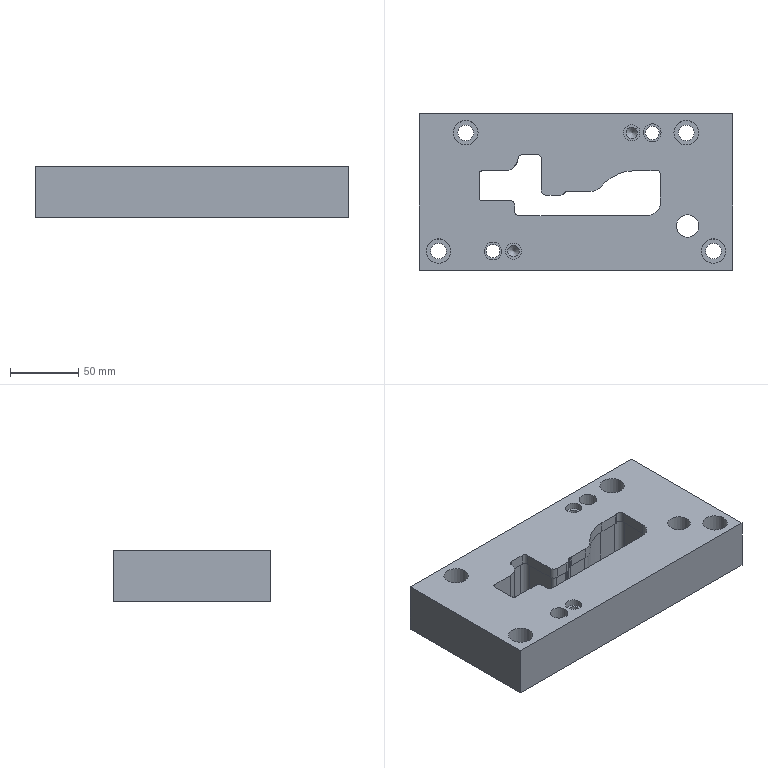Part | STEP file | lll_id278_x_t | 1 solid | 98 faces | box 230 x 115 x 38 mm | volume 809686 mm3 | cylinder 55 | plane 41 | cone 2 | commonest cylinder face diameters 6 x6 9 x4 11.509 x4 18.008 x4 20 x3 3 x2